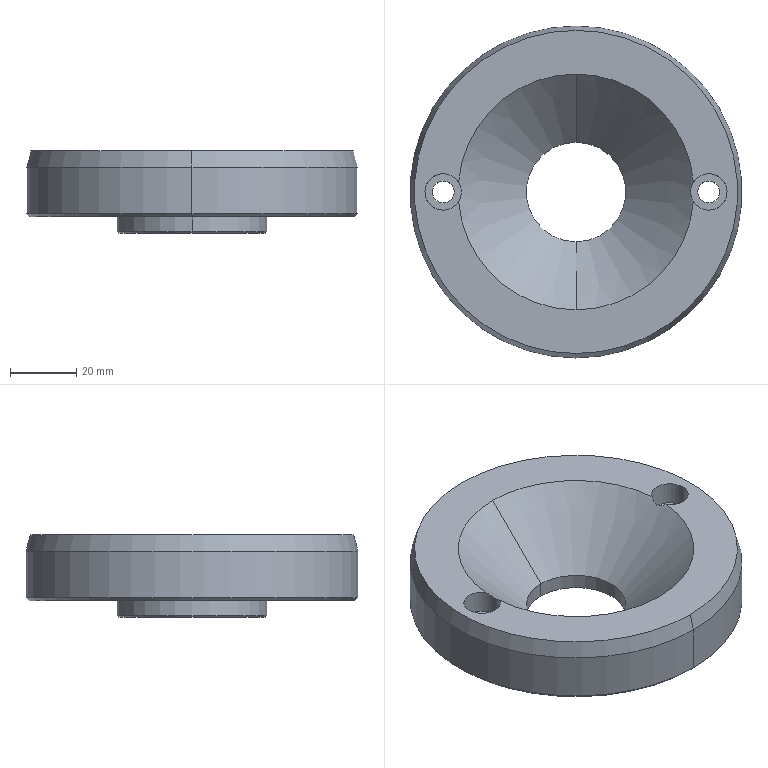Part | Creo | 1 solid | 27 faces | box 100 x 100 x 25 mm | volume 115102 mm3 | cylinder 14 | cone 8 | plane 5 | commonest cylinder face diameters 6.6 x4 11 x4 30 x2 45 x2 100 x2
STEP:
#1=CARTESIAN_POINT('',(0.,0.,0.));
#2=DIRECTION('',(0.,0.,1.));
#3=DIRECTION('',(1.,0.,0.));
#4=AXIS2_PLACEMENT_3D('',#1,#2,#3);
#5=CARTESIAN_POINT('',(34.5,60.,329.5));
#6=VERTEX_POINT('',#5);
#7=CARTESIAN_POINT('',(35.375,62.976,330.5));
#8=VERTEX_POINT('',#7);
#9=CARTESIAN_POINT('',(34.5,60.246,329.5));
#10=CARTESIAN_POINT('',(34.533,60.747,329.539));
#11=CARTESIAN_POINT('',(34.694,61.519,329.727));
#12=CARTESIAN_POINT('',(34.97,62.272,330.043));
#13=CARTESIAN_POINT('',(35.228,62.748,330.334));
#14=B_SPLINE_CURVE_WITH_KNOTS('',3,(#5,#9,#10,#11,#12,#13,#7),.UNSPECIFIED.,.F.,.F.,(4,1,1,1,4),(0.,0.25,0.5,0.75,1.),.UNSPECIFIED.);
#15=EDGE_CURVE('',#6,#8,#14,.T.);
#16=ORIENTED_EDGE('',*,*,#15,.T.);
#17=CARTESIAN_POINT('',(45.5,60.,330.5));
#18=VERTEX_POINT('',#17);
#19=CARTESIAN_POINT('',(40.,60.,330.5));
#20=DIRECTION('',(0.,0.,-1.));
#21=DIRECTION('',(-0.8409,0.5412,0.));
#22=AXIS2_PLACEMENT_3D('',#19,#20,#21);
#23=CIRCLE('',#22,5.5);
#24=EDGE_CURVE('',#8,#18,#23,.T.);
#25=ORIENTED_EDGE('',*,*,#24,.T.);
#26=CARTESIAN_POINT('',(45.5,60.,323.5));
#27=VERTEX_POINT('',#26);
#28=CARTESIAN_POINT('',(45.5,60.,330.5));
#29=DIRECTION('',(0.,0.,-1.));
#30=VECTOR('',#29,7.);
#31=LINE('',#28,#30);
#32=EDGE_CURVE('',#18,#27,#31,.T.);
#33=ORIENTED_EDGE('',*,*,#32,.T.);
#34=CARTESIAN_POINT('',(34.5,60.,323.5));
#35=VERTEX_POINT('',#34);
#36=CARTESIAN_POINT('',(40.,60.,323.5));
#37=DIRECTION('',(0.,0.,1.));
#38=DIRECTION('',(1.,0.,0.));
#39=AXIS2_PLACEMENT_3D('',#36,#37,#38);
#40=CIRCLE('',#39,5.5);
#41=EDGE_CURVE('',#27,#35,#40,.T.);
#42=ORIENTED_EDGE('',*,*,#41,.T.);
#43=CARTESIAN_POINT('',(34.5,60.,329.5));
#44=DIRECTION('',(0.,0.,-1.));
#45=VECTOR('',#44,6.);
#46=LINE('',#43,#45);
#47=EDGE_CURVE('',#6,#35,#46,.T.);
#48=ORIENTED_EDGE('',*,*,#47,.F.);
#49=EDGE_LOOP('',(#16,#25,#33,#42,#48));
#50=FACE_OUTER_BOUND('',#49,.F.);
#51=CARTESIAN_POINT('',(40.,60.,310.5));
#52=DIRECTION('',(0.,0.,-1.));
#53=DIRECTION('',(-1.,0.,0.));
#54=AXIS2_PLACEMENT_3D('',#51,#52,#53);
#55=CYLINDRICAL_SURFACE('',#54,5.5);
#56=ADVANCED_FACE('',(#50),#55,.F.);
#57=CARTESIAN_POINT('',(0.,75.,310.));
#58=VERTEX_POINT('',#57);
#59=CARTESIAN_POINT('',(0.,45.,310.));
#60=VERTEX_POINT('',#59);
#61=CARTESIAN_POINT('',(0.,60.,310.));
#62=DIRECTION('',(0.,0.,-1.));
#63=DIRECTION('',(0.,1.,0.));
#64=AXIS2_PLACEMENT_3D('',#61,#62,#63);
#65=CIRCLE('',#64,15.);
#66=EDGE_CURVE('',#58,#60,#65,.T.);
#67=ORIENTED_EDGE('',*,*,#66,.F.);
#68=CARTESIAN_POINT('',(0.,95.5,330.5));
#69=VERTEX_POINT('',#68);
#70=CARTESIAN_POINT('',(0.,95.5,330.5));
#71=DIRECTION('',(0.,-0.7071,-0.7071));
#72=VECTOR('',#71,28.991);
#73=LINE('',#70,#72);
#74=EDGE_CURVE('',#69,#58,#73,.T.);
#75=ORIENTED_EDGE('',*,*,#74,.F.);
#76=CARTESIAN_POINT('',(0.,60.,330.5));
#77=DIRECTION('',(0.,0.,-1.));
#78=DIRECTION('',(0.,1.,0.));
#79=AXIS2_PLACEMENT_3D('',#76,#77,#78);
#80=CIRCLE('',#79,35.5);
#81=EDGE_CURVE('',#69,#8,#80,.T.);
#82=ORIENTED_EDGE('',*,*,#81,.T.);
#83=ORIENTED_EDGE('',*,*,#15,.F.);
#84=CARTESIAN_POINT('',(35.375,57.024,330.5));
#85=VERTEX_POINT('',#84);
#86=CARTESIAN_POINT('',(34.5,60.,329.5));
#87=CARTESIAN_POINT('',(34.5,59.763,329.5));
#88=CARTESIAN_POINT('',(34.531,59.274,329.537));
#89=CARTESIAN_POINT('',(34.687,58.506,329.719));
#90=CARTESIAN_POINT('',(34.962,57.745,330.034));
#91=CARTESIAN_POINT('',(35.224,57.258,330.33));
#92=CARTESIAN_POINT('',(35.375,57.024,330.5));
#93=B_SPLINE_CURVE_WITH_KNOTS('',3,(#86,#87,#88,#89,#90,#91,#92),.UNSPECIFIED.,.F.,.F.,(4,1,1,1,4),(0.,0.25,0.5,0.75,1.),.UNSPECIFIED.);
#94=EDGE_CURVE('',#6,#85,#93,.T.);
#95=ORIENTED_EDGE('',*,*,#94,.T.);
#96=CARTESIAN_POINT('',(0.,24.5,330.5));
#97=VERTEX_POINT('',#96);
#98=CARTESIAN_POINT('',(0.,60.,330.5));
#99=DIRECTION('',(0.,0.,-1.));
#100=DIRECTION('',(0.9965,-0.08384,0.));
#101=AXIS2_PLACEMENT_3D('',#98,#99,#100);
#102=CIRCLE('',#101,35.5);
#103=EDGE_CURVE('',#85,#97,#102,.T.);
#104=ORIENTED_EDGE('',*,*,#103,.T.);
#105=CARTESIAN_POINT('',(0.,24.5,330.5));
#106=DIRECTION('',(0.,0.7071,-0.7071));
#107=VECTOR('',#106,28.991);
#108=LINE('',#105,#107);
#109=EDGE_CURVE('',#97,#60,#108,.T.);
#110=ORIENTED_EDGE('',*,*,#109,.T.);
#111=EDGE_LOOP('',(#67,#75,#82,#83,#95,#104,#110));
#112=FACE_OUTER_BOUND('',#111,.F.);
#113=CARTESIAN_POINT('',(0.,60.,320.25));
#114=DIRECTION('',(0.,0.,1.));
#115=DIRECTION('',(0.,-1.,0.));
#116=AXIS2_PLACEMENT_3D('',#113,#114,#115);
#117=CONICAL_SURFACE('',#116,25.25,45.);
#118=ADVANCED_FACE('',(#112),#117,.F.);
#119=CARTESIAN_POINT('',(0.,45.,305.5));
#120=VERTEX_POINT('',#119);
#121=CARTESIAN_POINT('',(0.,75.,305.5));
#122=VERTEX_POINT('',#121);
#123=CARTESIAN_POINT('',(0.,60.,305.5));
#124=DIRECTION('',(0.,0.,1.));
#125=DIRECTION('',(0.,-1.,0.));
#126=AXIS2_PLACEMENT_3D('',#123,#124,#125);
#127=CIRCLE('',#126,15.);
#128=EDGE_CURVE('',#120,#122,#127,.T.);
#129=ORIENTED_EDGE('',*,*,#128,.T.);
#130=CARTESIAN_POINT('',(0.,75.,310.));
#131=DIRECTION('',(0.,0.,-1.));
#132=VECTOR('',#131,4.5);
#133=LINE('',#130,#132);
#134=EDGE_CURVE('',#58,#122,#133,.T.);
#135=ORIENTED_EDGE('',*,*,#134,.F.);
#136=ORIENTED_EDGE('',*,*,#66,.T.);
#137=CARTESIAN_POINT('',(0.,45.,310.));
#138=DIRECTION('',(0.,0.,-1.));
#139=VECTOR('',#138,4.5);
#140=LINE('',#137,#139);
#141=EDGE_CURVE('',#60,#120,#140,.T.);
#142=ORIENTED_EDGE('',*,*,#141,.T.);
#143=EDGE_LOOP('',(#129,#135,#136,#142));
#144=FACE_OUTER_BOUND('',#143,.F.);
#145=CARTESIAN_POINT('',(0.,60.,330.5));
#146=DIRECTION('',(0.,0.,1.));
#147=DIRECTION('',(0.,-1.,0.));
#148=AXIS2_PLACEMENT_3D('',#145,#146,#147);
#149=CYLINDRICAL_SURFACE('',#148,15.);
#150=ADVANCED_FACE('',(#144),#149,.F.);
#151=CARTESIAN_POINT('',(0.,38.,305.5));
#152=VERTEX_POINT('',#151);
#153=CARTESIAN_POINT('',(0.,82.,305.5));
#154=VERTEX_POINT('',#153);
#155=CARTESIAN_POINT('',(0.,60.,305.5));
#156=DIRECTION('',(0.,0.,-1.));
#157=DIRECTION('',(0.,-1.,0.));
#158=AXIS2_PLACEMENT_3D('',#155,#156,#157);
#159=CIRCLE('',#158,22.);
#160=EDGE_CURVE('',#152,#154,#159,.T.);
#161=ORIENTED_EDGE('',*,*,#160,.F.);
#162=CARTESIAN_POINT('',(0.,60.,305.5));
#163=DIRECTION('',(0.,0.,-1.));
#164=DIRECTION('',(0.,1.,0.));
#165=AXIS2_PLACEMENT_3D('',#162,#163,#164);
#166=CIRCLE('',#165,22.);
#167=EDGE_CURVE('',#154,#152,#166,.T.);
#168=ORIENTED_EDGE('',*,*,#167,.F.);
#169=EDGE_LOOP('',(#161,#168));
#170=FACE_OUTER_BOUND('',#169,.F.);
#171=CARTESIAN_POINT('',(0.,60.,305.5));
#172=DIRECTION('',(0.,0.,1.));
#173=DIRECTION('',(0.,1.,0.));
#174=AXIS2_PLACEMENT_3D('',#171,#172,#173);
#175=CIRCLE('',#174,15.);
#176=EDGE_CURVE('',#122,#120,#175,.T.);
#177=ORIENTED_EDGE('',*,*,#176,.F.);
#178=ORIENTED_EDGE('',*,*,#128,.F.);
#179=EDGE_LOOP('',(#177,#178));
#180=FACE_BOUND('',#179,.F.);
#181=CARTESIAN_POINT('',(-0.5908,60.,305.5));
#182=DIRECTION('',(0.,0.,1.));
#183=DIRECTION('',(0.,-1.,0.));
#184=AXIS2_PLACEMENT_3D('',#181,#182,#183);
#185=PLANE('',#184);
#186=ADVANCED_FACE('',(#170,#180),#185,.F.);
#187=ORIENTED_EDGE('',*,*,#160,.T.);
#188=CARTESIAN_POINT('',(0.,82.5,306.));
#189=VERTEX_POINT('',#188);
#190=CARTESIAN_POINT('',(0.,82.5,306.));
#191=DIRECTION('',(0.,-0.7071,-0.7071));
#192=VECTOR('',#191,0.7071);
#193=LINE('',#190,#192);
#194=EDGE_CURVE('',#189,#154,#193,.T.);
#195=ORIENTED_EDGE('',*,*,#194,.F.);
#196=CARTESIAN_POINT('',(0.,37.5,306.));
#197=VERTEX_POINT('',#196);
#198=CARTESIAN_POINT('',(0.,60.,306.));
#199=DIRECTION('',(0.,0.,-1.));
#200=DIRECTION('',(0.,-1.,0.));
#201=AXIS2_PLACEMENT_3D('',#198,#199,#200);
#202=CIRCLE('',#201,22.5);
#203=EDGE_CURVE('',#197,#189,#202,.T.);
#204=ORIENTED_EDGE('',*,*,#203,.F.);
#205=CARTESIAN_POINT('',(0.,37.5,306.));
#206=DIRECTION('',(0.,0.7071,-0.7071));
#207=VECTOR('',#206,0.7071);
#208=LINE('',#205,#207);
#209=EDGE_CURVE('',#197,#152,#208,.T.);
#210=ORIENTED_EDGE('',*,*,#209,.T.);
#211=EDGE_LOOP('',(#187,#195,#204,#210));
#212=FACE_OUTER_BOUND('',#211,.F.);
#213=CARTESIAN_POINT('',(0.,60.,305.75));
#214=DIRECTION('',(0.,0.,1.));
#215=DIRECTION('',(0.,-1.,0.));
#216=AXIS2_PLACEMENT_3D('',#213,#214,#215);
#217=CONICAL_SURFACE('',#216,22.25,45.);
#218=ADVANCED_FACE('',(#212),#217,.T.);
#219=ORIENTED_EDGE('',*,*,#209,.F.);
#220=CARTESIAN_POINT('',(0.,60.,306.));
#221=DIRECTION('',(0.,0.,-1.));
#222=DIRECTION('',(0.,1.,0.));
#223=AXIS2_PLACEMENT_3D('',#220,#221,#222);
#224=CIRCLE('',#223,22.5);
#225=EDGE_CURVE('',#189,#197,#224,.T.);
#226=ORIENTED_EDGE('',*,*,#225,.F.);
#227=ORIENTED_EDGE('',*,*,#194,.T.);
#228=ORIENTED_EDGE('',*,*,#167,.T.);
#229=EDGE_LOOP('',(#219,#226,#227,#228));
#230=FACE_OUTER_BOUND('',#229,.F.);
#231=CARTESIAN_POINT('',(0.,60.,305.75));
#232=DIRECTION('',(0.,0.,1.));
#233=DIRECTION('',(0.,-1.,0.));
#234=AXIS2_PLACEMENT_3D('',#231,#232,#233);
#235=CONICAL_SURFACE('',#234,22.25,45.);
#236=ADVANCED_FACE('',(#230),#235,.T.);
#237=CARTESIAN_POINT('',(0.,37.5,310.5));
#238=VERTEX_POINT('',#237);
#239=CARTESIAN_POINT('',(0.,37.5,310.5));
#240=DIRECTION('',(0.,0.,-1.));
#241=VECTOR('',#240,4.5);
#242=LINE('',#239,#241);
#243=EDGE_CURVE('',#238,#197,#242,.T.);
#244=ORIENTED_EDGE('',*,*,#243,.F.);
#245=CARTESIAN_POINT('',(0.,82.5,310.5));
#246=VERTEX_POINT('',#245);
#247=CARTESIAN_POINT('',(0.,60.,310.5));
#248=DIRECTION('',(0.,0.,1.));
#249=DIRECTION('',(0.,-1.,0.));
#250=AXIS2_PLACEMENT_3D('',#247,#248,#249);
#251=CIRCLE('',#250,22.5);
#252=EDGE_CURVE('',#238,#246,#251,.T.);
#253=ORIENTED_EDGE('',*,*,#252,.T.);
#254=CARTESIAN_POINT('',(0.,82.5,310.5));
#255=DIRECTION('',(0.,0.,-1.));
#256=VECTOR('',#255,4.5);
#257=LINE('',#254,#256);
#258=EDGE_CURVE('',#246,#189,#257,.T.);
#259=ORIENTED_EDGE('',*,*,#258,.T.);
#260=ORIENTED_EDGE('',*,*,#225,.T.);
#261=EDGE_LOOP('',(#244,#253,#259,#260));
#262=FACE_OUTER_BOUND('',#261,.F.);
#263=CARTESIAN_POINT('',(0.,60.,330.5));
#264=DIRECTION('',(0.,0.,1.));
#265=DIRECTION('',(0.,-1.,0.));
#266=AXIS2_PLACEMENT_3D('',#263,#264,#265);
#267=CYLINDRICAL_SURFACE('',#266,22.5);
#268=ADVANCED_FACE('',(#262),#267,.T.);
#269=ORIENTED_EDGE('',*,*,#203,.T.);
#270=ORIENTED_EDGE('',*,*,#258,.F.);
#271=CARTESIAN_POINT('',(0.,60.,310.5));
#272=DIRECTION('',(0.,0.,1.));
#273=DIRECTION('',(0.,1.,0.));
#274=AXIS2_PLACEMENT_3D('',#271,#272,#273);
#275=CIRCLE('',#274,22.5);
#276=EDGE_CURVE('',#246,#238,#275,.T.);
#277=ORIENTED_EDGE('',*,*,#276,.T.);
#278=ORIENTED_EDGE('',*,*,#243,.T.);
#279=EDGE_LOOP('',(#269,#270,#277,#278));
#280=FACE_OUTER_BOUND('',#279,.F.);
#281=CARTESIAN_POINT('',(0.,60.,330.5));
#282=DIRECTION('',(0.,0.,1.));
#283=DIRECTION('',(0.,-1.,0.));
#284=AXIS2_PLACEMENT_3D('',#281,#282,#283);
#285=CYLINDRICAL_SURFACE('',#284,22.5);
#286=ADVANCED_FACE('',(#280),#285,.T.);
#287=CARTESIAN_POINT('',(0.,11.,310.5));
#288=VERTEX_POINT('',#287);
#289=CARTESIAN_POINT('',(0.,109.,310.5));
#290=VERTEX_POINT('',#289);
#291=CARTESIAN_POINT('',(0.,60.,310.5));
#292=DIRECTION('',(0.,0.,-1.));
#293=DIRECTION('',(0.,-1.,0.));
#294=AXIS2_PLACEMENT_3D('',#291,#292,#293);
#295=CIRCLE('',#294,49.);
#296=EDGE_CURVE('',#288,#290,#295,.T.);
#297=ORIENTED_EDGE('',*,*,#296,.F.);
#298=CARTESIAN_POINT('',(0.,60.,310.5));
#299=DIRECTION('',(0.,0.,-1.));
#300=DIRECTION('',(0.,1.,0.));
#301=AXIS2_PLACEMENT_3D('',#298,#299,#300);
#302=CIRCLE('',#301,49.);
#303=EDGE_CURVE('',#290,#288,#302,.T.);
#304=ORIENTED_EDGE('',*,*,#303,.F.);
#305=EDGE_LOOP('',(#297,#304));
#306=FACE_OUTER_BOUND('',#305,.F.);
#307=ORIENTED_EDGE('',*,*,#276,.F.);
#308=ORIENTED_EDGE('',*,*,#252,.F.);
#309=EDGE_LOOP('',(#307,#308));
#310=FACE_BOUND('',#309,.F.);
#311=CARTESIAN_POINT('',(-36.7,60.,310.5));
#312=VERTEX_POINT('',#311);
#313=CARTESIAN_POINT('',(-43.3,60.,310.5));
#314=VERTEX_POINT('',#313);
#315=CARTESIAN_POINT('',(-40.,60.,310.5));
#316=DIRECTION('',(0.,0.,1.));
#317=DIRECTION('',(1.,0.,0.));
#318=AXIS2_PLACEMENT_3D('',#315,#316,#317);
#319=CIRCLE('',#318,3.3);
#320=EDGE_CURVE('',#312,#314,#319,.T.);
#321=ORIENTED_EDGE('',*,*,#320,.F.);
#322=CARTESIAN_POINT('',(-40.,60.,310.5));
#323=DIRECTION('',(0.,0.,1.));
#324=DIRECTION('',(-1.,0.,0.));
#325=AXIS2_PLACEMENT_3D('',#322,#323,#324);
#326=CIRCLE('',#325,3.3);
#327=EDGE_CURVE('',#314,#312,#326,.T.);
#328=ORIENTED_EDGE('',*,*,#327,.F.);
#329=EDGE_LOOP('',(#321,#328));
#330=FACE_BOUND('',#329,.F.);
#331=CARTESIAN_POINT('',(36.7,60.,310.5));
#332=VERTEX_POINT('',#331);
#333=CARTESIAN_POINT('',(43.3,60.,310.5));
#334=VERTEX_POINT('',#333);
#335=CARTESIAN_POINT('',(40.,60.,310.5));
#336=DIRECTION('',(0.,0.,1.));
#337=DIRECTION('',(-1.,0.,0.));
#338=AXIS2_PLACEMENT_3D('',#335,#336,#337);
#339=CIRCLE('',#338,3.3);
#340=EDGE_CURVE('',#332,#334,#339,.T.);
#341=ORIENTED_EDGE('',*,*,#340,.F.);
#342=CARTESIAN_POINT('',(40.,60.,310.5));
#343=DIRECTION('',(0.,0.,1.));
#344=DIRECTION('',(1.,0.,0.));
#345=AXIS2_PLACEMENT_3D('',#342,#343,#344);
#346=CIRCLE('',#345,3.3);
#347=EDGE_CURVE('',#334,#332,#346,.T.);
#348=ORIENTED_EDGE('',*,*,#347,.F.);
#349=EDGE_LOOP('',(#341,#348));
#350=FACE_BOUND('',#349,.F.);
#351=CARTESIAN_POINT('',(-0.5908,60.,310.5));
#352=DIRECTION('',(0.,0.,-1.));
#353=DIRECTION('',(0.,1.,0.));
#354=AXIS2_PLACEMENT_3D('',#351,#352,#353);
#355=PLANE('',#354);
#356=ADVANCED_FACE('',(#306,#310,#330,#350),#355,.T.);
#357=CARTESIAN_POINT('',(-36.7,60.,323.5));
#358=VERTEX_POINT('',#357);
#359=CARTESIAN_POINT('',(-36.7,60.,323.5));
#360=DIRECTION('',(0.,0.,-1.));
#361=VECTOR('',#360,13.);
#362=LINE('',#359,#361);
#363=EDGE_CURVE('',#358,#312,#362,.T.);
#364=ORIENTED_EDGE('',*,*,#363,.T.);
#365=ORIENTED_EDGE('',*,*,#320,.T.);
#366=CARTESIAN_POINT('',(-43.3,60.,323.5));
#367=VERTEX_POINT('',#366);
#368=CARTESIAN_POINT('',(-43.3,60.,323.5));
#369=DIRECTION('',(0.,0.,-1.));
#370=VECTOR('',#369,13.);
#371=LINE('',#368,#370);
#372=EDGE_CURVE('',#367,#314,#371,.T.);
#373=ORIENTED_EDGE('',*,*,#372,.F.);
#374=CARTESIAN_POINT('',(-40.,60.,323.5));
#375=DIRECTION('',(0.,0.,-1.));
#376=DIRECTION('',(-1.,0.,0.));
#377=AXIS2_PLACEMENT_3D('',#374,#375,#376);
#378=CIRCLE('',#377,3.3);
#379=EDGE_CURVE('',#367,#358,#378,.T.);
#380=ORIENTED_EDGE('',*,*,#379,.T.);
#381=EDGE_LOOP('',(#364,#365,#373,#380));
#382=FACE_OUTER_BOUND('',#381,.F.);
#383=CARTESIAN_POINT('',(-40.,60.,310.5));
#384=DIRECTION('',(0.,0.,-1.));
#385=DIRECTION('',(1.,0.,0.));
#386=AXIS2_PLACEMENT_3D('',#383,#384,#385);
#387=CYLINDRICAL_SURFACE('',#386,3.3);
#388=ADVANCED_FACE('',(#382),#387,.F.);
#389=CARTESIAN_POINT('',(-40.,60.,323.5));
#390=DIRECTION('',(0.,0.,-1.));
#391=DIRECTION('',(1.,0.,0.));
#392=AXIS2_PLACEMENT_3D('',#389,#390,#391);
#393=CIRCLE('',#392,3.3);
#394=EDGE_CURVE('',#358,#367,#393,.T.);
#395=ORIENTED_EDGE('',*,*,#394,.T.);
#396=ORIENTED_EDGE('',*,*,#372,.T.);
#397=ORIENTED_EDGE('',*,*,#327,.T.);
#398=ORIENTED_EDGE('',*,*,#363,.F.);
#399=EDGE_LOOP('',(#395,#396,#397,#398));
#400=FACE_OUTER_BOUND('',#399,.F.);
#401=CARTESIAN_POINT('',(-40.,60.,310.5));
#402=DIRECTION('',(0.,0.,-1.));
#403=DIRECTION('',(1.,0.,0.));
#404=AXIS2_PLACEMENT_3D('',#401,#402,#403);
#405=CYLINDRICAL_SURFACE('',#404,3.3);
#406=ADVANCED_FACE('',(#400),#405,.F.);
#407=CARTESIAN_POINT('',(-34.5,60.,323.5));
#408=VERTEX_POINT('',#407);
#409=CARTESIAN_POINT('',(-45.5,60.,323.5));
#410=VERTEX_POINT('',#409);
#411=CARTESIAN_POINT('',(-40.,60.,323.5));
#412=DIRECTION('',(0.,0.,1.));
#413=DIRECTION('',(1.,0.,0.));
#414=AXIS2_PLACEMENT_3D('',#411,#412,#413);
#415=CIRCLE('',#414,5.5);
#416=EDGE_CURVE('',#408,#410,#415,.T.);
#417=ORIENTED_EDGE('',*,*,#416,.F.);
#418=CARTESIAN_POINT('',(-40.,60.,323.5));
#419=DIRECTION('',(0.,0.,1.));
#420=DIRECTION('',(-1.,0.,0.));
#421=AXIS2_PLACEMENT_3D('',#418,#419,#420);
#422=CIRCLE('',#421,5.5);
#423=EDGE_CURVE('',#410,#408,#422,.T.);
#424=ORIENTED_EDGE('',*,*,#423,.F.);
#425=EDGE_LOOP('',(#417,#424));
#426=FACE_OUTER_BOUND('',#425,.F.);
#427=ORIENTED_EDGE('',*,*,#379,.F.);
#428=ORIENTED_EDGE('',*,*,#394,.F.);
#429=EDGE_LOOP('',(#427,#428));
#430=FACE_BOUND('',#429,.F.);
#431=CARTESIAN_POINT('',(-0.5908,60.,323.5));
#432=DIRECTION('',(0.,0.,1.));
#433=DIRECTION('',(-1.,0.,0.));
#434=AXIS2_PLACEMENT_3D('',#431,#432,#433);
#435=PLANE('',#434);
#436=ADVANCED_FACE('',(#426,#430),#435,.T.);
#437=CARTESIAN_POINT('',(-34.5,60.,329.5));
#438=VERTEX_POINT('',#437);
#439=CARTESIAN_POINT('',(-34.5,60.,323.5));
#440=DIRECTION('',(0.,0.,1.));
#441=VECTOR('',#440,6.);
#442=LINE('',#439,#441);
#443=EDGE_CURVE('',#408,#438,#442,.T.);
#444=ORIENTED_EDGE('',*,*,#443,.F.);
#445=ORIENTED_EDGE('',*,*,#416,.T.);
#446=CARTESIAN_POINT('',(-45.5,60.,330.5));
#447=VERTEX_POINT('',#446);
#448=CARTESIAN_POINT('',(-45.5,60.,323.5));
#449=DIRECTION('',(0.,0.,1.));
#450=VECTOR('',#449,7.);
#451=LINE('',#448,#450);
#452=EDGE_CURVE('',#410,#447,#451,.T.);
#453=ORIENTED_EDGE('',*,*,#452,.T.);
#454=CARTESIAN_POINT('',(-35.375,62.976,330.5));
#455=VERTEX_POINT('',#454);
#456=CARTESIAN_POINT('',(-40.,60.,330.5));
#457=DIRECTION('',(0.,0.,-1.));
#458=DIRECTION('',(-1.,0.,0.));
#459=AXIS2_PLACEMENT_3D('',#456,#457,#458);
#460=CIRCLE('',#459,5.5);
#461=EDGE_CURVE('',#447,#455,#460,.T.);
#462=ORIENTED_EDGE('',*,*,#461,.T.);
#463=CARTESIAN_POINT('',(-34.5,60.,329.5));
#464=CARTESIAN_POINT('',(-34.5,60.237,329.5));
#465=CARTESIAN_POINT('',(-34.531,60.726,329.537));
#466=CARTESIAN_POINT('',(-34.687,61.494,329.719));
#467=CARTESIAN_POINT('',(-34.962,62.255,330.034));
#468=CARTESIAN_POINT('',(-35.224,62.742,330.33));
#469=CARTESIAN_POINT('',(-35.375,62.976,330.5));
#470=B_SPLINE_CURVE_WITH_KNOTS('',3,(#463,#464,#465,#466,#467,#468,#469),.UNSPECIFIED.,.F.,.F.,(4,1,1,1,4),(0.,0.25,0.5,0.75,1.),.UNSPECIFIED.);
#471=EDGE_CURVE('',#438,#455,#470,.T.);
#472=ORIENTED_EDGE('',*,*,#471,.F.);
#473=EDGE_LOOP('',(#444,#445,#453,#462,#472));
#474=FACE_OUTER_BOUND('',#473,.F.);
#475=CARTESIAN_POINT('',(-40.,60.,310.5));
#476=DIRECTION('',(0.,0.,-1.));
#477=DIRECTION('',(1.,0.,0.));
#478=AXIS2_PLACEMENT_3D('',#475,#476,#477);
#479=CYLINDRICAL_SURFACE('',#478,5.5);
#480=ADVANCED_FACE('',(#474),#479,.F.);
#481=CARTESIAN_POINT('',(-35.375,57.024,330.5));
#482=VERTEX_POINT('',#481);
#483=CARTESIAN_POINT('',(-34.5,59.754,329.5));
#484=CARTESIAN_POINT('',(-34.533,59.253,329.539));
#485=CARTESIAN_POINT('',(-34.694,58.481,329.727));
#486=CARTESIAN_POINT('',(-34.97,57.728,330.043));
#487=CARTESIAN_POINT('',(-35.228,57.252,330.334));
#488=B_SPLINE_CURVE_WITH_KNOTS('',3,(#437,#483,#484,#485,#486,#487,#481),.UNSPECIFIED.,.F.,.F.,(4,1,1,1,4),(0.,0.25,0.5,0.75,1.),.UNSPECIFIED.);
#489=EDGE_CURVE('',#438,#482,#488,.T.);
#490=ORIENTED_EDGE('',*,*,#489,.T.);
#491=CARTESIAN_POINT('',(-40.,60.,330.5));
#492=DIRECTION('',(0.,0.,-1.));
#493=DIRECTION('',(0.8409,-0.5412,0.));
#494=AXIS2_PLACEMENT_3D('',#491,#492,#493);
#495=CIRCLE('',#494,5.5);
#496=EDGE_CURVE('',#482,#447,#495,.T.);
#497=ORIENTED_EDGE('',*,*,#496,.T.);
#498=ORIENTED_EDGE('',*,*,#452,.F.);
#499=ORIENTED_EDGE('',*,*,#423,.T.);
#500=ORIENTED_EDGE('',*,*,#443,.T.);
#501=EDGE_LOOP('',(#490,#497,#498,#499,#500));
#502=FACE_OUTER_BOUND('',#501,.F.);
#503=CARTESIAN_POINT('',(-40.,60.,310.5));
#504=DIRECTION('',(0.,0.,-1.));
#505=DIRECTION('',(1.,0.,0.));
#506=AXIS2_PLACEMENT_3D('',#503,#504,#505);
#507=CYLINDRICAL_SURFACE('',#506,5.5);
#508=ADVANCED_FACE('',(#502),#507,.F.);
#509=ORIENTED_EDGE('',*,*,#109,.F.);
#510=CARTESIAN_POINT('',(0.,60.,330.5));
#511=DIRECTION('',(0.,0.,-1.));
#512=DIRECTION('',(0.,-1.,0.));
#513=AXIS2_PLACEMENT_3D('',#510,#511,#512);
#514=CIRCLE('',#513,35.5);
#515=EDGE_CURVE('',#97,#482,#514,.T.);
#516=ORIENTED_EDGE('',*,*,#515,.T.);
#517=ORIENTED_EDGE('',*,*,#489,.F.);
#518=ORIENTED_EDGE('',*,*,#471,.T.);
#519=CARTESIAN_POINT('',(0.,60.,330.5));
#520=DIRECTION('',(0.,0.,-1.));
#521=DIRECTION('',(-0.9965,0.08384,0.));
#522=AXIS2_PLACEMENT_3D('',#519,#520,#521);
#523=CIRCLE('',#522,35.5);
#524=EDGE_CURVE('',#455,#69,#523,.T.);
#525=ORIENTED_EDGE('',*,*,#524,.T.);
#526=ORIENTED_EDGE('',*,*,#74,.T.);
#527=CARTESIAN_POINT('',(0.,60.,310.));
#528=DIRECTION('',(0.,0.,-1.));
#529=DIRECTION('',(0.,-1.,0.));
#530=AXIS2_PLACEMENT_3D('',#527,#528,#529);
#531=CIRCLE('',#530,15.);
#532=EDGE_CURVE('',#60,#58,#531,.T.);
#533=ORIENTED_EDGE('',*,*,#532,.F.);
#534=EDGE_LOOP('',(#509,#516,#517,#518,#525,#526,#533));
#535=FACE_OUTER_BOUND('',#534,.F.);
#536=CARTESIAN_POINT('',(0.,60.,320.25));
#537=DIRECTION('',(0.,0.,1.));
#538=DIRECTION('',(0.,-1.,0.));
#539=AXIS2_PLACEMENT_3D('',#536,#537,#538);
#540=CONICAL_SURFACE('',#539,25.25,45.);
#541=ADVANCED_FACE('',(#535),#540,.F.);
#542=CARTESIAN_POINT('',(0.,11.34,330.5));
#543=VERTEX_POINT('',#542);
#544=CARTESIAN_POINT('',(0.,108.66,330.5));
#545=VERTEX_POINT('',#544);
#546=CARTESIAN_POINT('',(0.,60.,330.5));
#547=DIRECTION('',(0.,0.,1.));
#548=DIRECTION('',(0.,-1.,0.));
#549=AXIS2_PLACEMENT_3D('',#546,#547,#548);
#550=CIRCLE('',#549,48.66);
#551=EDGE_CURVE('',#543,#545,#550,.T.);
#552=ORIENTED_EDGE('',*,*,#551,.F.);
#553=CARTESIAN_POINT('',(0.,60.,330.5));
#554=DIRECTION('',(0.,0.,1.));
#555=DIRECTION('',(0.,1.,0.));
#556=AXIS2_PLACEMENT_3D('',#553,#554,#555);
#557=CIRCLE('',#556,48.66);
#558=EDGE_CURVE('',#545,#543,#557,.T.);
#559=ORIENTED_EDGE('',*,*,#558,.F.);
#560=EDGE_LOOP('',(#552,#559));
#561=FACE_OUTER_BOUND('',#560,.F.);
#562=ORIENTED_EDGE('',*,*,#81,.F.);
#563=ORIENTED_EDGE('',*,*,#524,.F.);
#564=ORIENTED_EDGE('',*,*,#461,.F.);
#565=ORIENTED_EDGE('',*,*,#496,.F.);
#566=ORIENTED_EDGE('',*,*,#515,.F.);
#567=ORIENTED_EDGE('',*,*,#103,.F.);
#568=CARTESIAN_POINT('',(40.,60.,330.5));
#569=DIRECTION('',(0.,0.,-1.));
#570=DIRECTION('',(1.,0.,0.));
#571=AXIS2_PLACEMENT_3D('',#568,#569,#570);
#572=CIRCLE('',#571,5.5);
#573=EDGE_CURVE('',#18,#85,#572,.T.);
#574=ORIENTED_EDGE('',*,*,#573,.F.);
#575=ORIENTED_EDGE('',*,*,#24,.F.);
#576=EDGE_LOOP('',(#562,#563,#564,#565,#566,#567,#574,#575));
#577=FACE_BOUND('',#576,.F.);
#578=CARTESIAN_POINT('',(-0.5908,60.,330.5));
#579=DIRECTION('',(0.,0.,1.));
#580=DIRECTION('',(0.,-1.,0.));
#581=AXIS2_PLACEMENT_3D('',#578,#579,#580);
#582=PLANE('',#581);
#583=ADVANCED_FACE('',(#561,#577),#582,.T.);
#584=CARTESIAN_POINT('',(0.,110.,325.5));
#585=VERTEX_POINT('',#584);
#586=CARTESIAN_POINT('',(0.,110.,325.5));
#587=DIRECTION('',(0.,-0.2588,0.9659));
#588=VECTOR('',#587,5.176);
#589=LINE('',#586,#588);
#590=EDGE_CURVE('',#585,#545,#589,.T.);
#591=ORIENTED_EDGE('',*,*,#590,.F.);
#592=CARTESIAN_POINT('',(0.,10.,325.5));
#593=VERTEX_POINT('',#592);
#594=CARTESIAN_POINT('',(0.,60.,325.5));
#595=DIRECTION('',(0.,0.,1.));
#596=DIRECTION('',(0.,-1.,0.));
#597=AXIS2_PLACEMENT_3D('',#594,#595,#596);
#598=CIRCLE('',#597,50.);
#599=EDGE_CURVE('',#593,#585,#598,.T.);
#600=ORIENTED_EDGE('',*,*,#599,.F.);
#601=CARTESIAN_POINT('',(0.,10.,325.5));
#602=DIRECTION('',(0.,0.2588,0.9659));
#603=VECTOR('',#602,5.176);
#604=LINE('',#601,#603);
#605=EDGE_CURVE('',#593,#543,#604,.T.);
#606=ORIENTED_EDGE('',*,*,#605,.T.);
#607=ORIENTED_EDGE('',*,*,#551,.T.);
#608=EDGE_LOOP('',(#591,#600,#606,#607));
#609=FACE_OUTER_BOUND('',#608,.F.);
#610=CARTESIAN_POINT('',(0.,60.,328.));
#611=DIRECTION('',(0.,0.,-1.));
#612=DIRECTION('',(0.,1.,0.));
#613=AXIS2_PLACEMENT_3D('',#610,#611,#612);
#614=CONICAL_SURFACE('',#613,49.33,15.);
#615=ADVANCED_FACE('',(#609),#614,.T.);
#616=ORIENTED_EDGE('',*,*,#558,.T.);
#617=ORIENTED_EDGE('',*,*,#605,.F.);
#618=CARTESIAN_POINT('',(0.,60.,325.5));
#619=DIRECTION('',(0.,0.,1.));
#620=DIRECTION('',(0.,1.,0.));
#621=AXIS2_PLACEMENT_3D('',#618,#619,#620);
#622=CIRCLE('',#621,50.);
#623=EDGE_CURVE('',#585,#593,#622,.T.);
#624=ORIENTED_EDGE('',*,*,#623,.F.);
#625=ORIENTED_EDGE('',*,*,#590,.T.);
#626=EDGE_LOOP('',(#616,#617,#624,#625));
#627=FACE_OUTER_BOUND('',#626,.F.);
#628=CARTESIAN_POINT('',(0.,60.,328.));
#629=DIRECTION('',(0.,0.,-1.));
#630=DIRECTION('',(0.,1.,0.));
#631=AXIS2_PLACEMENT_3D('',#628,#629,#630);
#632=CONICAL_SURFACE('',#631,49.33,15.);
#633=ADVANCED_FACE('',(#627),#632,.T.);
#634=CARTESIAN_POINT('',(0.,10.,311.5));
#635=VERTEX_POINT('',#634);
#636=CARTESIAN_POINT('',(0.,110.,311.5));
#637=VERTEX_POINT('',#636);
#638=CARTESIAN_POINT('',(0.,60.,311.5));
#639=DIRECTION('',(0.,0.,-1.));
#640=DIRECTION('',(0.,-1.,0.));
#641=AXIS2_PLACEMENT_3D('',#638,#639,#640);
#642=CIRCLE('',#641,50.);
#643=EDGE_CURVE('',#635,#637,#642,.T.);
#644=ORIENTED_EDGE('',*,*,#643,.T.);
#645=CARTESIAN_POINT('',(0.,110.,325.5));
#646=DIRECTION('',(0.,0.,-1.));
#647=VECTOR('',#646,14.);
#648=LINE('',#645,#647);
#649=EDGE_CURVE('',#585,#637,#648,.T.);
#650=ORIENTED_EDGE('',*,*,#649,.F.);
#651=ORIENTED_EDGE('',*,*,#623,.T.);
#652=CARTESIAN_POINT('',(0.,10.,325.5));
#653=DIRECTION('',(0.,0.,-1.));
#654=VECTOR('',#653,14.);
#655=LINE('',#652,#654);
#656=EDGE_CURVE('',#593,#635,#655,.T.);
#657=ORIENTED_EDGE('',*,*,#656,.T.);
#658=EDGE_LOOP('',(#644,#650,#651,#657));
#659=FACE_OUTER_BOUND('',#658,.F.);
#660=CARTESIAN_POINT('',(0.,60.,330.5));
#661=DIRECTION('',(0.,0.,1.));
#662=DIRECTION('',(0.,-1.,0.));
#663=AXIS2_PLACEMENT_3D('',#660,#661,#662);
#664=CYLINDRICAL_SURFACE('',#663,50.);
#665=ADVANCED_FACE('',(#659),#664,.T.);
#666=ORIENTED_EDGE('',*,*,#296,.T.);
#667=CARTESIAN_POINT('',(0.,110.,311.5));
#668=DIRECTION('',(0.,-0.7071,-0.7071));
#669=VECTOR('',#668,1.414);
#670=LINE('',#667,#669);
#671=EDGE_CURVE('',#637,#290,#670,.T.);
#672=ORIENTED_EDGE('',*,*,#671,.F.);
#673=ORIENTED_EDGE('',*,*,#643,.F.);
#674=CARTESIAN_POINT('',(0.,10.,311.5));
#675=DIRECTION('',(0.,0.7071,-0.7071));
#676=VECTOR('',#675,1.414);
#677=LINE('',#674,#676);
#678=EDGE_CURVE('',#635,#288,#677,.T.);
#679=ORIENTED_EDGE('',*,*,#678,.T.);
#680=EDGE_LOOP('',(#666,#672,#673,#679));
#681=FACE_OUTER_BOUND('',#680,.F.);
#682=CARTESIAN_POINT('',(0.,60.,311.));
#683=DIRECTION('',(0.,0.,1.));
#684=DIRECTION('',(0.,-1.,0.));
#685=AXIS2_PLACEMENT_3D('',#682,#683,#684);
#686=CONICAL_SURFACE('',#685,49.5,45.);
#687=ADVANCED_FACE('',(#681),#686,.T.);
#688=ORIENTED_EDGE('',*,*,#678,.F.);
#689=CARTESIAN_POINT('',(0.,60.,311.5));
#690=DIRECTION('',(0.,0.,-1.));
#691=DIRECTION('',(0.,1.,0.));
#692=AXIS2_PLACEMENT_3D('',#689,#690,#691);
#693=CIRCLE('',#692,50.);
#694=EDGE_CURVE('',#637,#635,#693,.T.);
#695=ORIENTED_EDGE('',*,*,#694,.F.);
#696=ORIENTED_EDGE('',*,*,#671,.T.);
#697=ORIENTED_EDGE('',*,*,#303,.T.);
#698=EDGE_LOOP('',(#688,#695,#696,#697));
#699=FACE_OUTER_BOUND('',#698,.F.);
#700=CARTESIAN_POINT('',(0.,60.,311.));
#701=DIRECTION('',(0.,0.,1.));
#702=DIRECTION('',(0.,-1.,0.));
#703=AXIS2_PLACEMENT_3D('',#700,#701,#702);
#704=CONICAL_SURFACE('',#703,49.5,45.);
#705=ADVANCED_FACE('',(#699),#704,.T.);
#706=ORIENTED_EDGE('',*,*,#656,.F.);
#707=ORIENTED_EDGE('',*,*,#599,.T.);
#708=ORIENTED_EDGE('',*,*,#649,.T.);
#709=ORIENTED_EDGE('',*,*,#694,.T.);
#710=EDGE_LOOP('',(#706,#707,#708,#709));
#711=FACE_OUTER_BOUND('',#710,.F.);
#712=CARTESIAN_POINT('',(0.,60.,330.5));
#713=DIRECTION('',(0.,0.,1.));
#714=DIRECTION('',(0.,-1.,0.));
#715=AXIS2_PLACEMENT_3D('',#712,#713,#714);
#716=CYLINDRICAL_SURFACE('',#715,50.);
#717=ADVANCED_FACE('',(#711),#716,.T.);
#718=ORIENTED_EDGE('',*,*,#47,.T.);
#719=CARTESIAN_POINT('',(40.,60.,323.5));
#720=DIRECTION('',(0.,0.,1.));
#721=DIRECTION('',(-1.,0.,0.));
#722=AXIS2_PLACEMENT_3D('',#719,#720,#721);
#723=CIRCLE('',#722,5.5);
#724=EDGE_CURVE('',#35,#27,#723,.T.);
#725=ORIENTED_EDGE('',*,*,#724,.T.);
#726=ORIENTED_EDGE('',*,*,#32,.F.);
#727=ORIENTED_EDGE('',*,*,#573,.T.);
#728=ORIENTED_EDGE('',*,*,#94,.F.);
#729=EDGE_LOOP('',(#718,#725,#726,#727,#728));
#730=FACE_OUTER_BOUND('',#729,.F.);
#731=CARTESIAN_POINT('',(40.,60.,310.5));
#732=DIRECTION('',(0.,0.,-1.));
#733=DIRECTION('',(-1.,0.,0.));
#734=AXIS2_PLACEMENT_3D('',#731,#732,#733);
#735=CYLINDRICAL_SURFACE('',#734,5.5);
#736=ADVANCED_FACE('',(#730),#735,.F.);
#737=ORIENTED_EDGE('',*,*,#724,.F.);
#738=ORIENTED_EDGE('',*,*,#41,.F.);
#739=EDGE_LOOP('',(#737,#738));
#740=FACE_OUTER_BOUND('',#739,.F.);
#741=CARTESIAN_POINT('',(43.3,60.,323.5));
#742=VERTEX_POINT('',#741);
#743=CARTESIAN_POINT('',(36.7,60.,323.5));
#744=VERTEX_POINT('',#743);
#745=CARTESIAN_POINT('',(40.,60.,323.5));
#746=DIRECTION('',(0.,0.,-1.));
#747=DIRECTION('',(1.,0.,0.));
#748=AXIS2_PLACEMENT_3D('',#745,#746,#747);
#749=CIRCLE('',#748,3.3);
#750=EDGE_CURVE('',#742,#744,#749,.T.);
#751=ORIENTED_EDGE('',*,*,#750,.F.);
#752=CARTESIAN_POINT('',(40.,60.,323.5));
#753=DIRECTION('',(0.,0.,-1.));
#754=DIRECTION('',(-1.,0.,0.));
#755=AXIS2_PLACEMENT_3D('',#752,#753,#754);
#756=CIRCLE('',#755,3.3);
#757=EDGE_CURVE('',#744,#742,#756,.T.);
#758=ORIENTED_EDGE('',*,*,#757,.F.);
#759=EDGE_LOOP('',(#751,#758));
#760=FACE_BOUND('',#759,.F.);
#761=CARTESIAN_POINT('',(0.5908,60.,323.5));
#762=DIRECTION('',(0.,0.,1.));
#763=DIRECTION('',(1.,0.,0.));
#764=AXIS2_PLACEMENT_3D('',#761,#762,#763);
#765=PLANE('',#764);
#766=ADVANCED_FACE('',(#740,#760),#765,.T.);
#767=CARTESIAN_POINT('',(36.7,60.,323.5));
#768=DIRECTION('',(0.,0.,-1.));
#769=VECTOR('',#768,13.);
#770=LINE('',#767,#769);
#771=EDGE_CURVE('',#744,#332,#770,.T.);
#772=ORIENTED_EDGE('',*,*,#771,.T.);
#773=ORIENTED_EDGE('',*,*,#340,.T.);
#774=CARTESIAN_POINT('',(43.3,60.,323.5));
#775=DIRECTION('',(0.,0.,-1.));
#776=VECTOR('',#775,13.);
#777=LINE('',#774,#776);
#778=EDGE_CURVE('',#742,#334,#777,.T.);
#779=ORIENTED_EDGE('',*,*,#778,.F.);
#780=ORIENTED_EDGE('',*,*,#750,.T.);
#781=EDGE_LOOP('',(#772,#773,#779,#780));
#782=FACE_OUTER_BOUND('',#781,.F.);
#783=CARTESIAN_POINT('',(40.,60.,310.5));
#784=DIRECTION('',(0.,0.,-1.));
#785=DIRECTION('',(-1.,0.,0.));
#786=AXIS2_PLACEMENT_3D('',#783,#784,#785);
#787=CYLINDRICAL_SURFACE('',#786,3.3);
#788=ADVANCED_FACE('',(#782),#787,.F.);
#789=ORIENTED_EDGE('',*,*,#757,.T.);
#790=ORIENTED_EDGE('',*,*,#778,.T.);
#791=ORIENTED_EDGE('',*,*,#347,.T.);
#792=ORIENTED_EDGE('',*,*,#771,.F.);
#793=EDGE_LOOP('',(#789,#790,#791,#792));
#794=FACE_OUTER_BOUND('',#793,.F.);
#795=CARTESIAN_POINT('',(40.,60.,310.5));
#796=DIRECTION('',(0.,0.,-1.));
#797=DIRECTION('',(-1.,0.,0.));
#798=AXIS2_PLACEMENT_3D('',#795,#796,#797);
#799=CYLINDRICAL_SURFACE('',#798,3.3);
#800=ADVANCED_FACE('',(#794),#799,.F.);
#801=ORIENTED_EDGE('',*,*,#141,.F.);
#802=ORIENTED_EDGE('',*,*,#532,.T.);
#803=ORIENTED_EDGE('',*,*,#134,.T.);
#804=ORIENTED_EDGE('',*,*,#176,.T.);
#805=EDGE_LOOP('',(#801,#802,#803,#804));
#806=FACE_OUTER_BOUND('',#805,.F.);
#807=CARTESIAN_POINT('',(0.,60.,330.5));
#808=DIRECTION('',(0.,0.,1.));
#809=DIRECTION('',(0.,-1.,0.));
#810=AXIS2_PLACEMENT_3D('',#807,#808,#809);
#811=CYLINDRICAL_SURFACE('',#810,15.);
#812=ADVANCED_FACE('',(#806),#811,.F.);
#813=CLOSED_SHELL('',(#56,#118,#150,#186,#218,#236,#268,#286,#356,#388,#406,#436,#480,#508,#541,#583,#615,#633,#665,#687,#705,#717,#736,#766,#788,#800,#812));
#814=MANIFOLD_SOLID_BREP('',#813);
#815=(LENGTH_UNIT()NAMED_UNIT(*)SI_UNIT(.MILLI.,.METRE.));
#816=UNCERTAINTY_MEASURE_WITH_UNIT(LENGTH_MEASURE(0.01436),#815,'','');
#817=(NAMED_UNIT(*)PLANE_ANGLE_UNIT()SI_UNIT($,.RADIAN.));
#818=PLANE_ANGLE_MEASURE_WITH_UNIT(PLANE_ANGLE_MEASURE(0.01745),#817);
#819=(CONVERSION_BASED_UNIT('DEGREE',#818)NAMED_UNIT(*)PLANE_ANGLE_UNIT());
#820=(NAMED_UNIT(*)SI_UNIT($,.STERADIAN.)SOLID_ANGLE_UNIT());
#821=(GEOMETRIC_REPRESENTATION_CONTEXT(3)GLOBAL_UNCERTAINTY_ASSIGNED_CONTEXT((#816))GLOBAL_UNIT_ASSIGNED_CONTEXT((#815,#819,#820))REPRESENTATION_CONTEXT('',''));
#822=ADVANCED_BREP_SHAPE_REPRESENTATION('',(#4,#814),#821);